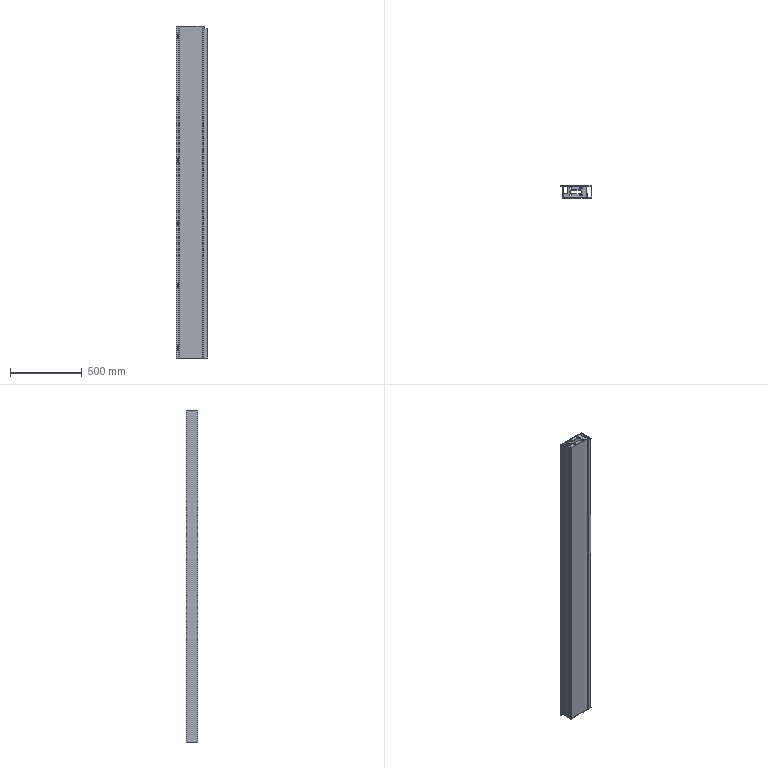Part | 5 solids | 154 faces | box 220 x 80 x 2316 mm | volume 3362845 mm3 | plane 88 | cylinder 66 | commonest cylinder face diameters 10 x24 8 x19 2 x9 6 x8 25 x6